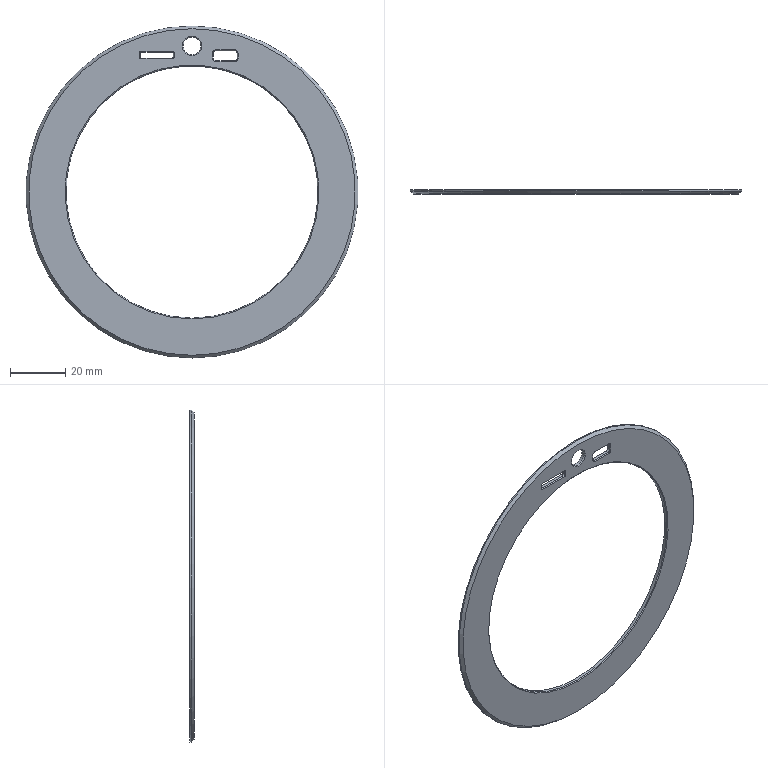CAM job | NX | 3-axis milling | part box 119.8 x 1.45 x 119.8 mm | stock box 145 x 36.45 x 145 mm
Tools:
number,name,description,diameter,corner_radius,flute_length,length,flutes
3,C3.0,Milling Tool-5 Parameters,3.0,0.0,15.0,30.0,2
0,C5.0,Milling Tool-5 Parameters,5.0,0.0,50.0,100.0,2
Operations:
program,operation,operation_type,tool,method,geometry_group,spindle_rpm,surface_speed,feed_per_tooth,feed_cut,feed_plunge,cut_length_mm,path_length_mm,cut_time_min,machine_time_min
PROGRAM,PROFILE_3D,PlanarMilling,C5.0,METHOD,WORKPIECE,5000.0,78.54,0.07,700.0,80.0,398.59,398.59,0.5716,0.5716
PROGRAM,PROFILE_3D_COPY,PlanarMilling,C5.0,METHOD,WORKPIECE,7000.0,109.0,0.1071,1500.0,100.0,286.329,286.329,0.1909,0.1909
PROGRAM,PROFILE_3D_COPY_COPY,PlanarMilling,C3.0,METHOD,WORKPIECE,7000.0,109.0,0.1071,1500.0,100.0,21.045,21.045,0.014,0.014
PROGRAM,PROFILE_3D_COPY_COPY_COPY,PlanarMilling,C3.0,METHOD,WORKPIECE,7000.0,109.0,0.1071,1500.0,100.0,19.894,19.894,0.0133,0.0133
PROGRAM,PROFILE_3D_COPY_COPY_COPY_COPY,PlanarMilling,C3.0,METHOD,WORKPIECE,7000.0,109.0,0.1071,1500.0,100.0,25.5,25.5,0.017,0.017